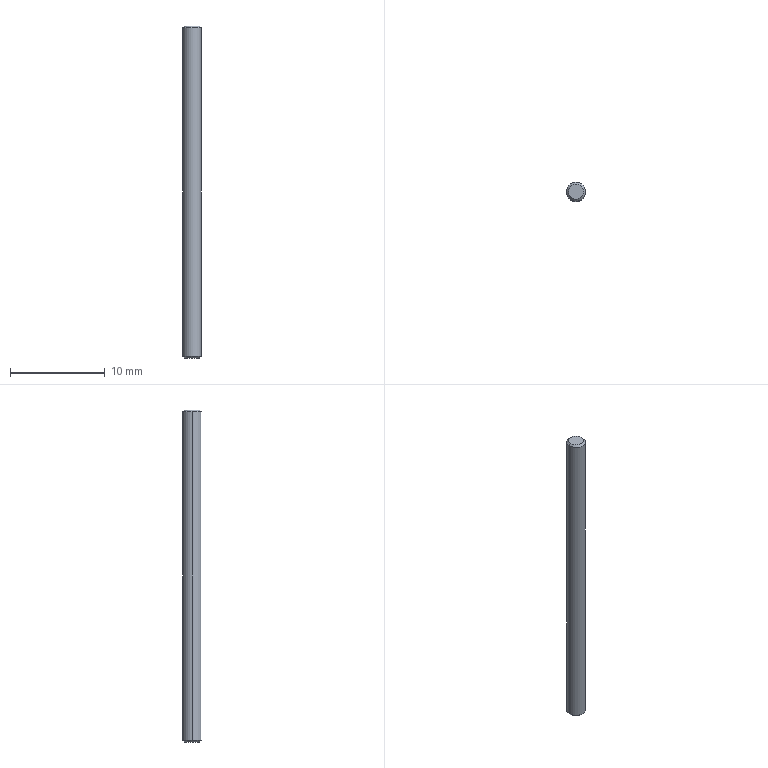Part | SolidWorks | features Chamfer 1, Extrusion 1, RefAxis 1 | 1 solid | 8 faces | box 2 x 2 x 35 mm | volume 109.721 mm3 | cone 4 | cylinder 2 | plane 2 | commonest cylinder face diameters 2 x2
STEP:
#1=CARTESIAN_POINT('',(0.8,0.,17.5));
#2=VERTEX_POINT('',#1);
#3=CARTESIAN_POINT('',(-0.8,0.,17.5));
#4=VERTEX_POINT('',#3);
#5=CARTESIAN_POINT('',(0.,0.,17.5));
#6=DIRECTION('',(0.,0.,1.));
#7=DIRECTION('',(1.,0.,0.));
#8=AXIS2_PLACEMENT_3D('',#5,#6,#7);
#9=CIRCLE('',#8,0.8);
#10=EDGE_CURVE('',#2,#4,#9,.T.);
#11=ORIENTED_EDGE('',*,*,#10,.F.);
#12=CARTESIAN_POINT('',(1.,0.,17.3));
#13=VERTEX_POINT('',#12);
#14=CARTESIAN_POINT('',(0.8,0.,17.5));
#15=DIRECTION('',(0.7071,0.,-0.7071));
#16=VECTOR('',#15,1000.);
#17=LINE('',#14,#16);
#18=EDGE_CURVE('',#2,#13,#17,.T.);
#19=ORIENTED_EDGE('',*,*,#18,.T.);
#20=CARTESIAN_POINT('',(-1.,0.,17.3));
#21=VERTEX_POINT('',#20);
#22=CARTESIAN_POINT('',(0.,0.,17.3));
#23=DIRECTION('',(0.,0.,-1.));
#24=DIRECTION('',(1.,0.,0.));
#25=AXIS2_PLACEMENT_3D('',#22,#23,#24);
#26=CIRCLE('',#25,1.);
#27=EDGE_CURVE('',#21,#13,#26,.T.);
#28=ORIENTED_EDGE('',*,*,#27,.F.);
#29=CARTESIAN_POINT('',(-0.8,0.,17.5));
#30=DIRECTION('',(-0.7071,0.,-0.7071));
#31=VECTOR('',#30,1000.);
#32=LINE('',#29,#31);
#33=EDGE_CURVE('',#4,#21,#32,.T.);
#34=ORIENTED_EDGE('',*,*,#33,.F.);
#35=EDGE_LOOP('',(#11,#19,#28,#34));
#36=FACE_OUTER_BOUND('',#35,.T.);
#37=CARTESIAN_POINT('',(0.,0.,17.5));
#38=DIRECTION('',(0.,0.,-1.));
#39=DIRECTION('',(-1.,0.,0.));
#40=AXIS2_PLACEMENT_3D('',#37,#38,#39);
#41=CONICAL_SURFACE('',#40,0.8,0.7854);
#42=ADVANCED_FACE('',(#36),#41,.T.);
#43=CARTESIAN_POINT('',(-0.8,0.,-17.5));
#44=VERTEX_POINT('',#43);
#45=CARTESIAN_POINT('',(0.8,0.,-17.5));
#46=VERTEX_POINT('',#45);
#47=CARTESIAN_POINT('',(0.,0.,-17.5));
#48=DIRECTION('',(0.,0.,-1.));
#49=DIRECTION('',(1.,0.,0.));
#50=AXIS2_PLACEMENT_3D('',#47,#48,#49);
#51=CIRCLE('',#50,0.8);
#52=EDGE_CURVE('',#44,#46,#51,.T.);
#53=ORIENTED_EDGE('',*,*,#52,.F.);
#54=CARTESIAN_POINT('',(-1.,0.,-17.3));
#55=VERTEX_POINT('',#54);
#56=CARTESIAN_POINT('',(-1.,0.,-17.3));
#57=DIRECTION('',(-0.7071,0.,0.7071));
#58=VECTOR('',#57,1000.);
#59=LINE('',#56,#58);
#60=EDGE_CURVE('',#44,#55,#59,.T.);
#61=ORIENTED_EDGE('',*,*,#60,.T.);
#62=CARTESIAN_POINT('',(1.,0.,-17.3));
#63=VERTEX_POINT('',#62);
#64=CARTESIAN_POINT('',(0.,0.,-17.3));
#65=DIRECTION('',(0.,0.,1.));
#66=DIRECTION('',(1.,0.,0.));
#67=AXIS2_PLACEMENT_3D('',#64,#65,#66);
#68=CIRCLE('',#67,1.);
#69=EDGE_CURVE('',#63,#55,#68,.T.);
#70=ORIENTED_EDGE('',*,*,#69,.F.);
#71=CARTESIAN_POINT('',(1.,0.,-17.3));
#72=DIRECTION('',(0.7071,0.,0.7071));
#73=VECTOR('',#72,1000.);
#74=LINE('',#71,#73);
#75=EDGE_CURVE('',#46,#63,#74,.T.);
#76=ORIENTED_EDGE('',*,*,#75,.F.);
#77=EDGE_LOOP('',(#53,#61,#70,#76));
#78=FACE_OUTER_BOUND('',#77,.T.);
#79=CARTESIAN_POINT('',(0.,0.,-17.3));
#80=DIRECTION('',(0.,0.,1.));
#81=DIRECTION('',(1.,0.,0.));
#82=AXIS2_PLACEMENT_3D('',#79,#80,#81);
#83=CONICAL_SURFACE('',#82,1.,0.7854);
#84=ADVANCED_FACE('',(#78),#83,.T.);
#85=ORIENTED_EDGE('',*,*,#27,.T.);
#86=CARTESIAN_POINT('',(1.,0.,17.5));
#87=DIRECTION('',(0.,0.,-1.));
#88=VECTOR('',#87,1000.);
#89=LINE('',#86,#88);
#90=EDGE_CURVE('',#13,#63,#89,.T.);
#91=ORIENTED_EDGE('',*,*,#90,.T.);
#92=ORIENTED_EDGE('',*,*,#69,.T.);
#93=CARTESIAN_POINT('',(-1.,0.,17.5));
#94=DIRECTION('',(0.,0.,-1.));
#95=VECTOR('',#94,1000.);
#96=LINE('',#93,#95);
#97=EDGE_CURVE('',#21,#55,#96,.T.);
#98=ORIENTED_EDGE('',*,*,#97,.F.);
#99=EDGE_LOOP('',(#85,#91,#92,#98));
#100=FACE_OUTER_BOUND('',#99,.T.);
#101=CARTESIAN_POINT('',(0.,0.,17.5));
#102=DIRECTION('',(0.,0.,-1.));
#103=DIRECTION('',(-1.,0.,0.));
#104=AXIS2_PLACEMENT_3D('',#101,#102,#103);
#105=CYLINDRICAL_SURFACE('',#104,1.);
#106=ADVANCED_FACE('',(#100),#105,.T.);
#107=ORIENTED_EDGE('',*,*,#90,.F.);
#108=CARTESIAN_POINT('',(0.,0.,17.3));
#109=DIRECTION('',(0.,0.,-1.));
#110=DIRECTION('',(1.,0.,0.));
#111=AXIS2_PLACEMENT_3D('',#108,#109,#110);
#112=CIRCLE('',#111,1.);
#113=EDGE_CURVE('',#13,#21,#112,.T.);
#114=ORIENTED_EDGE('',*,*,#113,.T.);
#115=ORIENTED_EDGE('',*,*,#97,.T.);
#116=CARTESIAN_POINT('',(0.,0.,-17.3));
#117=DIRECTION('',(0.,0.,1.));
#118=DIRECTION('',(1.,0.,0.));
#119=AXIS2_PLACEMENT_3D('',#116,#117,#118);
#120=CIRCLE('',#119,1.);
#121=EDGE_CURVE('',#55,#63,#120,.T.);
#122=ORIENTED_EDGE('',*,*,#121,.T.);
#123=EDGE_LOOP('',(#107,#114,#115,#122));
#124=FACE_OUTER_BOUND('',#123,.T.);
#125=CARTESIAN_POINT('',(0.,0.,17.5));
#126=DIRECTION('',(0.,0.,-1.));
#127=DIRECTION('',(-1.,0.,0.));
#128=AXIS2_PLACEMENT_3D('',#125,#126,#127);
#129=CYLINDRICAL_SURFACE('',#128,1.);
#130=ADVANCED_FACE('',(#124),#129,.T.);
#131=CARTESIAN_POINT('',(0.,0.,17.5));
#132=DIRECTION('',(0.,0.,1.));
#133=DIRECTION('',(1.,0.,0.));
#134=AXIS2_PLACEMENT_3D('',#131,#132,#133);
#135=CIRCLE('',#134,0.8);
#136=EDGE_CURVE('',#4,#2,#135,.T.);
#137=ORIENTED_EDGE('',*,*,#136,.T.);
#138=ORIENTED_EDGE('',*,*,#10,.T.);
#139=EDGE_LOOP('',(#137,#138));
#140=FACE_OUTER_BOUND('',#139,.T.);
#141=CARTESIAN_POINT('',(0.,0.,17.5));
#142=DIRECTION('',(0.,0.,1.));
#143=DIRECTION('',(1.,0.,0.));
#144=AXIS2_PLACEMENT_3D('',#141,#142,#143);
#145=PLANE('',#144);
#146=ADVANCED_FACE('',(#140),#145,.T.);
#147=CARTESIAN_POINT('',(0.,0.,-17.5));
#148=DIRECTION('',(0.,0.,-1.));
#149=DIRECTION('',(1.,0.,0.));
#150=AXIS2_PLACEMENT_3D('',#147,#148,#149);
#151=CIRCLE('',#150,0.8);
#152=EDGE_CURVE('',#46,#44,#151,.T.);
#153=ORIENTED_EDGE('',*,*,#152,.T.);
#154=ORIENTED_EDGE('',*,*,#52,.T.);
#155=EDGE_LOOP('',(#153,#154));
#156=FACE_OUTER_BOUND('',#155,.T.);
#157=CARTESIAN_POINT('',(0.,0.,-17.5));
#158=DIRECTION('',(0.,0.,1.));
#159=DIRECTION('',(1.,0.,0.));
#160=AXIS2_PLACEMENT_3D('',#157,#158,#159);
#161=PLANE('',#160);
#162=ADVANCED_FACE('',(#156),#161,.F.);
#163=ORIENTED_EDGE('',*,*,#60,.F.);
#164=ORIENTED_EDGE('',*,*,#152,.F.);
#165=ORIENTED_EDGE('',*,*,#75,.T.);
#166=ORIENTED_EDGE('',*,*,#121,.F.);
#167=EDGE_LOOP('',(#163,#164,#165,#166));
#168=FACE_OUTER_BOUND('',#167,.T.);
#169=CARTESIAN_POINT('',(0.,0.,-17.3));
#170=DIRECTION('',(0.,0.,1.));
#171=DIRECTION('',(1.,0.,0.));
#172=AXIS2_PLACEMENT_3D('',#169,#170,#171);
#173=CONICAL_SURFACE('',#172,1.,0.7854);
#174=ADVANCED_FACE('',(#168),#173,.T.);
#175=ORIENTED_EDGE('',*,*,#18,.F.);
#176=ORIENTED_EDGE('',*,*,#136,.F.);
#177=ORIENTED_EDGE('',*,*,#33,.T.);
#178=ORIENTED_EDGE('',*,*,#113,.F.);
#179=EDGE_LOOP('',(#175,#176,#177,#178));
#180=FACE_OUTER_BOUND('',#179,.T.);
#181=CARTESIAN_POINT('',(0.,0.,17.5));
#182=DIRECTION('',(0.,0.,-1.));
#183=DIRECTION('',(-1.,0.,0.));
#184=AXIS2_PLACEMENT_3D('',#181,#182,#183);
#185=CONICAL_SURFACE('',#184,0.8,0.7854);
#186=ADVANCED_FACE('',(#180),#185,.T.);
#187=CLOSED_SHELL('',(#42,#84,#106,#130,#146,#162,#174,#186));
#188=MANIFOLD_SOLID_BREP('',#187);
#189=CARTESIAN_POINT('',(0.,0.,0.));
#190=DIRECTION('',(0.,0.,1.));
#191=DIRECTION('',(1.,0.,0.));
#192=AXIS2_PLACEMENT_3D('',#189,#190,#191);
#193=(LENGTH_UNIT()NAMED_UNIT(*)SI_UNIT(.MILLI.,.METRE.));
#194=UNCERTAINTY_MEASURE_WITH_UNIT(LENGTH_MEASURE(0.00001),#193,'','');
#195=(NAMED_UNIT(*)PLANE_ANGLE_UNIT()SI_UNIT($,.RADIAN.));
#196=(NAMED_UNIT(*)SI_UNIT($,.STERADIAN.)SOLID_ANGLE_UNIT());
#197=(GEOMETRIC_REPRESENTATION_CONTEXT(3)GLOBAL_UNCERTAINTY_ASSIGNED_CONTEXT((#194))GLOBAL_UNIT_ASSIGNED_CONTEXT((#193,#195,#196))REPRESENTATION_CONTEXT('',''));
#198=ADVANCED_BREP_SHAPE_REPRESENTATION('',(#188,#192),#197);